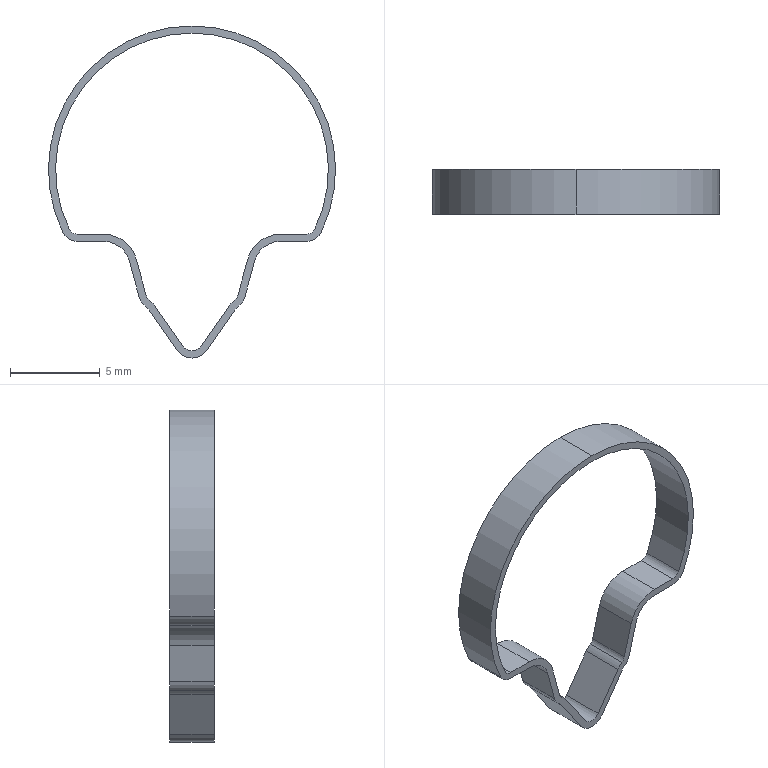Part | SolidWorks | features BaseBody 1 | 1 solid | 36 faces | box 16 x 2.5 x 18.5 mm | volume 53.347 mm3 | cylinder 22 | plane 14 | commonest cylinder face diameters 1 x4 1.8 x4 2 x3 2.8 x2 3 x2 3.8 x2
STEP:
#1=CARTESIAN_POINT('',(-7.197,-1.25,-3.493));
#2=VERTEX_POINT('',#1);
#3=CARTESIAN_POINT('',(0.,-1.25,8.));
#4=VERTEX_POINT('',#3);
#5=CARTESIAN_POINT('',(0.,-1.25,0.));
#6=DIRECTION('',(0.,1.,0.));
#7=DIRECTION('',(0.,0.,1.));
#8=AXIS2_PLACEMENT_3D('',#5,#6,#7);
#9=CIRCLE('',#8,8.);
#10=EDGE_CURVE('',#2,#4,#9,.T.);
#11=ORIENTED_EDGE('',*,*,#10,.T.);
#12=CARTESIAN_POINT('',(0.,1.25,8.));
#13=VERTEX_POINT('',#12);
#14=CARTESIAN_POINT('',(0.,-1.25,8.));
#15=DIRECTION('',(0.,1.,0.));
#16=VECTOR('',#15,1000.);
#17=LINE('',#14,#16);
#18=EDGE_CURVE('',#4,#13,#17,.T.);
#19=ORIENTED_EDGE('',*,*,#18,.T.);
#20=CARTESIAN_POINT('',(-7.197,1.25,-3.493));
#21=VERTEX_POINT('',#20);
#22=CARTESIAN_POINT('',(0.,1.25,0.));
#23=DIRECTION('',(0.,-1.,0.));
#24=DIRECTION('',(0.,0.,1.));
#25=AXIS2_PLACEMENT_3D('',#22,#23,#24);
#26=CIRCLE('',#25,8.);
#27=EDGE_CURVE('',#13,#21,#26,.T.);
#28=ORIENTED_EDGE('',*,*,#27,.T.);
#29=CARTESIAN_POINT('',(-7.197,-1.25,-3.493));
#30=DIRECTION('',(0.,-1.,0.));
#31=VECTOR('',#30,1000.);
#32=LINE('',#29,#31);
#33=EDGE_CURVE('',#21,#2,#32,.T.);
#34=ORIENTED_EDGE('',*,*,#33,.T.);
#35=EDGE_LOOP('',(#11,#19,#28,#34));
#36=FACE_OUTER_BOUND('',#35,.T.);
#37=CARTESIAN_POINT('',(0.,-1.25,0.));
#38=DIRECTION('',(0.,1.,0.));
#39=DIRECTION('',(0.,0.,1.));
#40=AXIS2_PLACEMENT_3D('',#37,#38,#39);
#41=CYLINDRICAL_SURFACE('',#40,8.);
#42=ADVANCED_FACE('',(#36),#41,.T.);
#43=CARTESIAN_POINT('',(6.837,-1.25,-3.318));
#44=VERTEX_POINT('',#43);
#45=CARTESIAN_POINT('',(0.,-1.25,7.6));
#46=VERTEX_POINT('',#45);
#47=CARTESIAN_POINT('',(0.,-1.25,0.));
#48=DIRECTION('',(0.,-1.,0.));
#49=DIRECTION('',(0.,0.,1.));
#50=AXIS2_PLACEMENT_3D('',#47,#48,#49);
#51=CIRCLE('',#50,7.6);
#52=EDGE_CURVE('',#44,#46,#51,.T.);
#53=ORIENTED_EDGE('',*,*,#52,.T.);
#54=CARTESIAN_POINT('',(0.,1.25,7.6));
#55=VERTEX_POINT('',#54);
#56=CARTESIAN_POINT('',(0.,-1.25,7.6));
#57=DIRECTION('',(0.,1.,0.));
#58=VECTOR('',#57,1000.);
#59=LINE('',#56,#58);
#60=EDGE_CURVE('',#46,#55,#59,.T.);
#61=ORIENTED_EDGE('',*,*,#60,.T.);
#62=CARTESIAN_POINT('',(6.837,1.25,-3.318));
#63=VERTEX_POINT('',#62);
#64=CARTESIAN_POINT('',(0.,1.25,0.));
#65=DIRECTION('',(0.,-1.,0.));
#66=DIRECTION('',(0.,0.,1.));
#67=AXIS2_PLACEMENT_3D('',#64,#65,#66);
#68=CIRCLE('',#67,7.6);
#69=EDGE_CURVE('',#63,#55,#68,.T.);
#70=ORIENTED_EDGE('',*,*,#69,.F.);
#71=CARTESIAN_POINT('',(6.837,-1.25,-3.318));
#72=DIRECTION('',(0.,1.,0.));
#73=VECTOR('',#72,1000.);
#74=LINE('',#71,#73);
#75=EDGE_CURVE('',#44,#63,#74,.T.);
#76=ORIENTED_EDGE('',*,*,#75,.F.);
#77=EDGE_LOOP('',(#53,#61,#70,#76));
#78=FACE_OUTER_BOUND('',#77,.T.);
#79=CARTESIAN_POINT('',(0.,-1.25,0.));
#80=DIRECTION('',(0.,1.,0.));
#81=DIRECTION('',(0.,0.,1.));
#82=AXIS2_PLACEMENT_3D('',#79,#80,#81);
#83=CYLINDRICAL_SURFACE('',#82,7.6);
#84=ADVANCED_FACE('',(#78),#83,.F.);
#85=ORIENTED_EDGE('',*,*,#18,.F.);
#86=CARTESIAN_POINT('',(7.197,-1.25,-3.493));
#87=VERTEX_POINT('',#86);
#88=CARTESIAN_POINT('',(0.,-1.25,0.));
#89=DIRECTION('',(0.,1.,0.));
#90=DIRECTION('',(0.,0.,1.));
#91=AXIS2_PLACEMENT_3D('',#88,#89,#90);
#92=CIRCLE('',#91,8.);
#93=EDGE_CURVE('',#4,#87,#92,.T.);
#94=ORIENTED_EDGE('',*,*,#93,.T.);
#95=CARTESIAN_POINT('',(7.197,1.25,-3.493));
#96=VERTEX_POINT('',#95);
#97=CARTESIAN_POINT('',(7.197,-1.25,-3.493));
#98=DIRECTION('',(0.,1.,0.));
#99=VECTOR('',#98,1000.);
#100=LINE('',#97,#99);
#101=EDGE_CURVE('',#87,#96,#100,.T.);
#102=ORIENTED_EDGE('',*,*,#101,.T.);
#103=CARTESIAN_POINT('',(0.,1.25,0.));
#104=DIRECTION('',(0.,-1.,0.));
#105=DIRECTION('',(0.,0.,1.));
#106=AXIS2_PLACEMENT_3D('',#103,#104,#105);
#107=CIRCLE('',#106,8.);
#108=EDGE_CURVE('',#96,#13,#107,.T.);
#109=ORIENTED_EDGE('',*,*,#108,.T.);
#110=EDGE_LOOP('',(#85,#94,#102,#109));
#111=FACE_OUTER_BOUND('',#110,.T.);
#112=CARTESIAN_POINT('',(0.,-1.25,0.));
#113=DIRECTION('',(0.,1.,0.));
#114=DIRECTION('',(0.,0.,1.));
#115=AXIS2_PLACEMENT_3D('',#112,#113,#114);
#116=CYLINDRICAL_SURFACE('',#115,8.);
#117=ADVANCED_FACE('',(#111),#116,.T.);
#118=CARTESIAN_POINT('',(6.387,-1.25,-4.));
#119=VERTEX_POINT('',#118);
#120=CARTESIAN_POINT('',(6.387,1.25,-4.));
#121=VERTEX_POINT('',#120);
#122=CARTESIAN_POINT('',(6.387,-4.509,-4.));
#123=DIRECTION('',(0.,1.,0.));
#124=VECTOR('',#123,1000.);
#125=LINE('',#122,#124);
#126=EDGE_CURVE('',#119,#121,#125,.T.);
#127=ORIENTED_EDGE('',*,*,#126,.T.);
#128=CARTESIAN_POINT('',(6.387,1.25,-3.1));
#129=DIRECTION('',(0.,-1.,0.));
#130=DIRECTION('',(0.,0.,1.));
#131=AXIS2_PLACEMENT_3D('',#128,#129,#130);
#132=CIRCLE('',#131,0.9);
#133=EDGE_CURVE('',#121,#96,#132,.T.);
#134=ORIENTED_EDGE('',*,*,#133,.T.);
#135=ORIENTED_EDGE('',*,*,#101,.F.);
#136=CARTESIAN_POINT('',(6.387,-1.25,-3.1));
#137=DIRECTION('',(0.,1.,0.));
#138=DIRECTION('',(0.,0.,1.));
#139=AXIS2_PLACEMENT_3D('',#136,#137,#138);
#140=CIRCLE('',#139,0.9);
#141=EDGE_CURVE('',#87,#119,#140,.T.);
#142=ORIENTED_EDGE('',*,*,#141,.T.);
#143=EDGE_LOOP('',(#127,#134,#135,#142));
#144=FACE_OUTER_BOUND('',#143,.T.);
#145=CARTESIAN_POINT('',(6.387,-4.509,-3.1));
#146=DIRECTION('',(0.,1.,0.));
#147=DIRECTION('',(0.,0.,1.));
#148=AXIS2_PLACEMENT_3D('',#145,#146,#147);
#149=CYLINDRICAL_SURFACE('',#148,0.9);
#150=ADVANCED_FACE('',(#144),#149,.T.);
#151=CARTESIAN_POINT('',(-4.931,-1.25,-3.6));
#152=VERTEX_POINT('',#151);
#153=CARTESIAN_POINT('',(-6.387,-1.25,-3.6));
#154=VERTEX_POINT('',#153);
#155=CARTESIAN_POINT('',(-7.144,-1.25,-3.6));
#156=DIRECTION('',(-1.,0.,0.));
#157=VECTOR('',#156,1000.);
#158=LINE('',#155,#157);
#159=EDGE_CURVE('',#152,#154,#158,.T.);
#160=ORIENTED_EDGE('',*,*,#159,.T.);
#161=CARTESIAN_POINT('',(-6.837,-1.25,-3.318));
#162=VERTEX_POINT('',#161);
#163=CARTESIAN_POINT('',(-6.387,-1.25,-3.1));
#164=DIRECTION('',(0.,1.,0.));
#165=DIRECTION('',(0.,0.,-1.));
#166=AXIS2_PLACEMENT_3D('',#163,#164,#165);
#167=CIRCLE('',#166,0.5);
#168=EDGE_CURVE('',#154,#162,#167,.T.);
#169=ORIENTED_EDGE('',*,*,#168,.T.);
#170=CARTESIAN_POINT('',(0.,-1.25,0.));
#171=DIRECTION('',(0.,-1.,0.));
#172=DIRECTION('',(0.,0.,1.));
#173=AXIS2_PLACEMENT_3D('',#170,#171,#172);
#174=CIRCLE('',#173,7.6);
#175=EDGE_CURVE('',#46,#162,#174,.T.);
#176=ORIENTED_EDGE('',*,*,#175,.F.);
#177=ORIENTED_EDGE('',*,*,#52,.F.);
#178=CARTESIAN_POINT('',(6.387,-1.25,-3.6));
#179=VERTEX_POINT('',#178);
#180=CARTESIAN_POINT('',(6.387,-1.25,-3.1));
#181=DIRECTION('',(0.,1.,0.));
#182=DIRECTION('',(0.,0.,1.));
#183=AXIS2_PLACEMENT_3D('',#180,#181,#182);
#184=CIRCLE('',#183,0.5);
#185=EDGE_CURVE('',#44,#179,#184,.T.);
#186=ORIENTED_EDGE('',*,*,#185,.T.);
#187=CARTESIAN_POINT('',(4.931,-1.25,-3.6));
#188=VERTEX_POINT('',#187);
#189=CARTESIAN_POINT('',(7.144,-1.25,-3.6));
#190=DIRECTION('',(1.,0.,0.));
#191=VECTOR('',#190,1000.);
#192=LINE('',#189,#191);
#193=EDGE_CURVE('',#188,#179,#192,.T.);
#194=ORIENTED_EDGE('',*,*,#193,.F.);
#195=CARTESIAN_POINT('',(3.096,-1.25,-5.008));
#196=VERTEX_POINT('',#195);
#197=CARTESIAN_POINT('',(4.931,-1.25,-5.5));
#198=DIRECTION('',(0.,1.,0.));
#199=DIRECTION('',(0.,0.,-1.));
#200=AXIS2_PLACEMENT_3D('',#197,#198,#199);
#201=CIRCLE('',#200,1.9);
#202=EDGE_CURVE('',#196,#188,#201,.T.);
#203=ORIENTED_EDGE('',*,*,#202,.F.);
#204=CARTESIAN_POINT('',(2.559,-1.25,-7.011));
#205=VERTEX_POINT('',#204);
#206=CARTESIAN_POINT('',(2.559,-1.25,-7.011));
#207=DIRECTION('',(0.2588,0.,0.9659));
#208=VECTOR('',#207,1000.);
#209=LINE('',#206,#208);
#210=EDGE_CURVE('',#205,#196,#209,.T.);
#211=ORIENTED_EDGE('',*,*,#210,.F.);
#212=CARTESIAN_POINT('',(2.373,-1.25,-7.284));
#213=VERTEX_POINT('',#212);
#214=CARTESIAN_POINT('',(2.076,-1.25,-6.882));
#215=DIRECTION('',(0.,1.,0.));
#216=DIRECTION('',(0.,0.,-1.));
#217=AXIS2_PLACEMENT_3D('',#214,#215,#216);
#218=CIRCLE('',#217,0.5);
#219=EDGE_CURVE('',#205,#213,#218,.T.);
#220=ORIENTED_EDGE('',*,*,#219,.T.);
#221=CARTESIAN_POINT('',(2.058,-1.25,-7.607));
#222=VERTEX_POINT('',#221);
#223=CARTESIAN_POINT('',(3.205,-1.25,-8.41));
#224=DIRECTION('',(0.,1.,0.));
#225=DIRECTION('',(0.,0.,1.));
#226=AXIS2_PLACEMENT_3D('',#223,#224,#225);
#227=CIRCLE('',#226,1.4);
#228=EDGE_CURVE('',#222,#213,#227,.T.);
#229=ORIENTED_EDGE('',*,*,#228,.F.);
#230=CARTESIAN_POINT('',(0.4915,-1.25,-9.844));
#231=VERTEX_POINT('',#230);
#232=CARTESIAN_POINT('',(0.4915,-1.25,-9.844));
#233=DIRECTION('',(0.5736,0.,0.8192));
#234=VECTOR('',#233,1000.);
#235=LINE('',#232,#234);
#236=EDGE_CURVE('',#231,#222,#235,.T.);
#237=ORIENTED_EDGE('',*,*,#236,.F.);
#238=CARTESIAN_POINT('',(-0.4915,-1.25,-9.844));
#239=VERTEX_POINT('',#238);
#240=CARTESIAN_POINT('',(0.,-1.25,-9.5));
#241=DIRECTION('',(0.,1.,0.));
#242=DIRECTION('',(0.,0.,1.));
#243=AXIS2_PLACEMENT_3D('',#240,#241,#242);
#244=CIRCLE('',#243,0.6);
#245=EDGE_CURVE('',#231,#239,#244,.T.);
#246=ORIENTED_EDGE('',*,*,#245,.T.);
#247=CARTESIAN_POINT('',(-2.058,-1.25,-7.607));
#248=VERTEX_POINT('',#247);
#249=CARTESIAN_POINT('',(-2.058,-1.25,-7.607));
#250=DIRECTION('',(0.5736,0.,-0.8192));
#251=VECTOR('',#250,1000.);
#252=LINE('',#249,#251);
#253=EDGE_CURVE('',#248,#239,#252,.T.);
#254=ORIENTED_EDGE('',*,*,#253,.F.);
#255=CARTESIAN_POINT('',(-2.373,-1.25,-7.284));
#256=VERTEX_POINT('',#255);
#257=CARTESIAN_POINT('',(-3.205,-1.25,-8.41));
#258=DIRECTION('',(0.,1.,0.));
#259=DIRECTION('',(0.,0.,1.));
#260=AXIS2_PLACEMENT_3D('',#257,#258,#259);
#261=CIRCLE('',#260,1.4);
#262=EDGE_CURVE('',#256,#248,#261,.T.);
#263=ORIENTED_EDGE('',*,*,#262,.F.);
#264=CARTESIAN_POINT('',(-2.559,-1.25,-7.011));
#265=VERTEX_POINT('',#264);
#266=CARTESIAN_POINT('',(-2.076,-1.25,-6.882));
#267=DIRECTION('',(0.,1.,0.));
#268=DIRECTION('',(0.,0.,1.));
#269=AXIS2_PLACEMENT_3D('',#266,#267,#268);
#270=CIRCLE('',#269,0.5);
#271=EDGE_CURVE('',#256,#265,#270,.T.);
#272=ORIENTED_EDGE('',*,*,#271,.T.);
#273=CARTESIAN_POINT('',(-3.096,-1.25,-5.008));
#274=VERTEX_POINT('',#273);
#275=CARTESIAN_POINT('',(-3.096,-1.25,-5.008));
#276=DIRECTION('',(0.2588,0.,-0.9659));
#277=VECTOR('',#276,1000.);
#278=LINE('',#275,#277);
#279=EDGE_CURVE('',#274,#265,#278,.T.);
#280=ORIENTED_EDGE('',*,*,#279,.F.);
#281=CARTESIAN_POINT('',(-4.931,-1.25,-5.5));
#282=DIRECTION('',(0.,1.,0.));
#283=DIRECTION('',(0.,0.,1.));
#284=AXIS2_PLACEMENT_3D('',#281,#282,#283);
#285=CIRCLE('',#284,1.9);
#286=EDGE_CURVE('',#152,#274,#285,.T.);
#287=ORIENTED_EDGE('',*,*,#286,.F.);
#288=EDGE_LOOP('',(#160,#169,#176,#177,#186,#194,#203,#211,#220,#229,#237,#246,#254,#263,#272,#280,#287));
#289=FACE_BOUND('',#288,.T.);
#290=CARTESIAN_POINT('',(-0.8192,-1.25,-10.074));
#291=VERTEX_POINT('',#290);
#292=CARTESIAN_POINT('',(-2.386,-1.25,-7.837));
#293=VERTEX_POINT('',#292);
#294=CARTESIAN_POINT('',(-0.8192,-1.25,-10.074));
#295=DIRECTION('',(-0.5736,0.,0.8192));
#296=VECTOR('',#295,1000.);
#297=LINE('',#294,#296);
#298=EDGE_CURVE('',#291,#293,#297,.T.);
#299=ORIENTED_EDGE('',*,*,#298,.F.);
#300=CARTESIAN_POINT('',(0.8192,-1.25,-10.074));
#301=VERTEX_POINT('',#300);
#302=CARTESIAN_POINT('',(0.,-1.25,-9.5));
#303=DIRECTION('',(0.,1.,0.));
#304=DIRECTION('',(0.,0.,1.));
#305=AXIS2_PLACEMENT_3D('',#302,#303,#304);
#306=CIRCLE('',#305,1.);
#307=EDGE_CURVE('',#301,#291,#306,.T.);
#308=ORIENTED_EDGE('',*,*,#307,.F.);
#309=CARTESIAN_POINT('',(2.386,-1.25,-7.837));
#310=VERTEX_POINT('',#309);
#311=CARTESIAN_POINT('',(2.386,-1.25,-7.837));
#312=DIRECTION('',(-0.5736,0.,-0.8192));
#313=VECTOR('',#312,1000.);
#314=LINE('',#311,#313);
#315=EDGE_CURVE('',#310,#301,#314,.T.);
#316=ORIENTED_EDGE('',*,*,#315,.F.);
#317=CARTESIAN_POINT('',(2.611,-1.25,-7.606));
#318=VERTEX_POINT('',#317);
#319=CARTESIAN_POINT('',(3.205,-1.25,-8.41));
#320=DIRECTION('',(0.,1.,0.));
#321=DIRECTION('',(0.,0.,1.));
#322=AXIS2_PLACEMENT_3D('',#319,#320,#321);
#323=CIRCLE('',#322,1.);
#324=EDGE_CURVE('',#310,#318,#323,.T.);
#325=ORIENTED_EDGE('',*,*,#324,.T.);
#326=CARTESIAN_POINT('',(2.945,-1.25,-7.115));
#327=VERTEX_POINT('',#326);
#328=CARTESIAN_POINT('',(2.076,-1.25,-6.882));
#329=DIRECTION('',(0.,1.,0.));
#330=DIRECTION('',(0.,0.,-1.));
#331=AXIS2_PLACEMENT_3D('',#328,#329,#330);
#332=CIRCLE('',#331,0.9);
#333=EDGE_CURVE('',#327,#318,#332,.T.);
#334=ORIENTED_EDGE('',*,*,#333,.F.);
#335=CARTESIAN_POINT('',(3.482,-1.25,-5.112));
#336=VERTEX_POINT('',#335);
#337=CARTESIAN_POINT('',(3.482,-1.25,-5.112));
#338=DIRECTION('',(-0.2588,0.,-0.9659));
#339=VECTOR('',#338,1000.);
#340=LINE('',#337,#339);
#341=EDGE_CURVE('',#336,#327,#340,.T.);
#342=ORIENTED_EDGE('',*,*,#341,.F.);
#343=CARTESIAN_POINT('',(4.931,-1.25,-4.));
#344=VERTEX_POINT('',#343);
#345=CARTESIAN_POINT('',(4.931,-1.25,-5.5));
#346=DIRECTION('',(0.,-1.,0.));
#347=DIRECTION('',(0.,0.,-1.));
#348=AXIS2_PLACEMENT_3D('',#345,#346,#347);
#349=CIRCLE('',#348,1.5);
#350=EDGE_CURVE('',#344,#336,#349,.T.);
#351=ORIENTED_EDGE('',*,*,#350,.F.);
#352=CARTESIAN_POINT('',(0.,-1.25,-4.));
#353=DIRECTION('',(-1.,0.,0.));
#354=VECTOR('',#353,1000.);
#355=LINE('',#352,#354);
#356=EDGE_CURVE('',#119,#344,#355,.T.);
#357=ORIENTED_EDGE('',*,*,#356,.F.);
#358=ORIENTED_EDGE('',*,*,#141,.F.);
#359=ORIENTED_EDGE('',*,*,#93,.F.);
#360=ORIENTED_EDGE('',*,*,#10,.F.);
#361=CARTESIAN_POINT('',(-6.387,-1.25,-4.));
#362=VERTEX_POINT('',#361);
#363=CARTESIAN_POINT('',(-6.387,-1.25,-3.1));
#364=DIRECTION('',(0.,1.,0.));
#365=DIRECTION('',(0.,0.,-1.));
#366=AXIS2_PLACEMENT_3D('',#363,#364,#365);
#367=CIRCLE('',#366,0.9);
#368=EDGE_CURVE('',#362,#2,#367,.T.);
#369=ORIENTED_EDGE('',*,*,#368,.F.);
#370=CARTESIAN_POINT('',(-4.931,-1.25,-4.));
#371=VERTEX_POINT('',#370);
#372=CARTESIAN_POINT('',(-4.931,-1.25,-4.));
#373=DIRECTION('',(1.,0.,0.));
#374=VECTOR('',#373,1000.);
#375=LINE('',#372,#374);
#376=EDGE_CURVE('',#362,#371,#375,.T.);
#377=ORIENTED_EDGE('',*,*,#376,.T.);
#378=CARTESIAN_POINT('',(-3.482,-1.25,-5.112));
#379=VERTEX_POINT('',#378);
#380=CARTESIAN_POINT('',(-4.931,-1.25,-5.5));
#381=DIRECTION('',(0.,-1.,0.));
#382=DIRECTION('',(0.,0.,1.));
#383=AXIS2_PLACEMENT_3D('',#380,#381,#382);
#384=CIRCLE('',#383,1.5);
#385=EDGE_CURVE('',#379,#371,#384,.T.);
#386=ORIENTED_EDGE('',*,*,#385,.F.);
#387=CARTESIAN_POINT('',(-2.945,-1.25,-7.115));
#388=VERTEX_POINT('',#387);
#389=CARTESIAN_POINT('',(-2.945,-1.25,-7.115));
#390=DIRECTION('',(-0.2588,0.,0.9659));
#391=VECTOR('',#390,1000.);
#392=LINE('',#389,#391);
#393=EDGE_CURVE('',#388,#379,#392,.T.);
#394=ORIENTED_EDGE('',*,*,#393,.F.);
#395=CARTESIAN_POINT('',(-2.611,-1.25,-7.606));
#396=VERTEX_POINT('',#395);
#397=CARTESIAN_POINT('',(-2.076,-1.25,-6.882));
#398=DIRECTION('',(0.,1.,0.));
#399=DIRECTION('',(0.,0.,1.));
#400=AXIS2_PLACEMENT_3D('',#397,#398,#399);
#401=CIRCLE('',#400,0.9);
#402=EDGE_CURVE('',#396,#388,#401,.T.);
#403=ORIENTED_EDGE('',*,*,#402,.F.);
#404=CARTESIAN_POINT('',(-3.205,-1.25,-8.41));
#405=DIRECTION('',(0.,1.,0.));
#406=DIRECTION('',(0.,0.,1.));
#407=AXIS2_PLACEMENT_3D('',#404,#405,#406);
#408=CIRCLE('',#407,1.);
#409=EDGE_CURVE('',#396,#293,#408,.T.);
#410=ORIENTED_EDGE('',*,*,#409,.T.);
#411=EDGE_LOOP('',(#299,#308,#316,#325,#334,#342,#351,#357,#358,#359,#360,#369,#377,#386,#394,#403,#410));
#412=FACE_OUTER_BOUND('',#411,.T.);
#413=CARTESIAN_POINT('',(0.,-1.25,0.));
#414=DIRECTION('',(0.,1.,0.));
#415=DIRECTION('',(0.,0.,1.));
#416=AXIS2_PLACEMENT_3D('',#413,#414,#415);
#417=PLANE('',#416);
#418=ADVANCED_FACE('',(#289,#412),#417,.F.);
#419=CARTESIAN_POINT('',(-6.387,1.25,-4.));
#420=VERTEX_POINT('',#419);
#421=CARTESIAN_POINT('',(-6.387,4.509,-4.));
#422=DIRECTION('',(0.,-1.,0.));
#423=VECTOR('',#422,1000.);
#424=LINE('',#421,#423);
#425=EDGE_CURVE('',#420,#362,#424,.T.);
#426=ORIENTED_EDGE('',*,*,#425,.T.);
#427=ORIENTED_EDGE('',*,*,#368,.T.);
#428=ORIENTED_EDGE('',*,*,#33,.F.);
#429=CARTESIAN_POINT('',(-6.387,1.25,-3.1));
#430=DIRECTION('',(0.,-1.,0.));
#431=DIRECTION('',(0.,0.,-1.));
#432=AXIS2_PLACEMENT_3D('',#429,#430,#431);
#433=CIRCLE('',#432,0.9);
#434=EDGE_CURVE('',#21,#420,#433,.T.);
#435=ORIENTED_EDGE('',*,*,#434,.T.);
#436=EDGE_LOOP('',(#426,#427,#428,#435));
#437=FACE_OUTER_BOUND('',#436,.T.);
#438=CARTESIAN_POINT('',(-6.387,4.509,-3.1));
#439=DIRECTION('',(0.,-1.,0.));
#440=DIRECTION('',(0.,0.,-1.));
#441=AXIS2_PLACEMENT_3D('',#438,#439,#440);
#442=CYLINDRICAL_SURFACE('',#441,0.9);
#443=ADVANCED_FACE('',(#437),#442,.T.);
#444=CARTESIAN_POINT('',(-2.559,1.25,-7.011));
#445=VERTEX_POINT('',#444);
#446=CARTESIAN_POINT('',(-2.373,1.25,-7.284));
#447=VERTEX_POINT('',#446);
#448=CARTESIAN_POINT('',(-2.076,1.25,-6.882));
#449=DIRECTION('',(0.,-1.,0.));
#450=DIRECTION('',(0.,0.,1.));
#451=AXIS2_PLACEMENT_3D('',#448,#449,#450);
#452=CIRCLE('',#451,0.5);
#453=EDGE_CURVE('',#445,#447,#452,.T.);
#454=ORIENTED_EDGE('',*,*,#453,.T.);
#455=CARTESIAN_POINT('',(-2.058,1.25,-7.607));
#456=VERTEX_POINT('',#455);
#457=CARTESIAN_POINT('',(-3.205,1.25,-8.41));
#458=DIRECTION('',(0.,-1.,0.));
#459=DIRECTION('',(0.,0.,1.));
#460=AXIS2_PLACEMENT_3D('',#457,#458,#459);
#461=CIRCLE('',#460,1.4);
#462=EDGE_CURVE('',#456,#447,#461,.T.);
#463=ORIENTED_EDGE('',*,*,#462,.F.);
#464=CARTESIAN_POINT('',(-0.4915,1.25,-9.844));
#465=VERTEX_POINT('',#464);
#466=CARTESIAN_POINT('',(-2.058,1.25,-7.607));
#467=DIRECTION('',(0.5736,0.,-0.8192));
#468=VECTOR('',#467,1000.);
#469=LINE('',#466,#468);
#470=EDGE_CURVE('',#456,#465,#469,.T.);
#471=ORIENTED_EDGE('',*,*,#470,.T.);
#472=CARTESIAN_POINT('',(0.4915,1.25,-9.844));
#473=VERTEX_POINT('',#472);
#474=CARTESIAN_POINT('',(0.,1.25,-9.5));
#475=DIRECTION('',(0.,-1.,0.));
#476=DIRECTION('',(0.,0.,1.));
#477=AXIS2_PLACEMENT_3D('',#474,#475,#476);
#478=CIRCLE('',#477,0.6);
#479=EDGE_CURVE('',#465,#473,#478,.T.);
#480=ORIENTED_EDGE('',*,*,#479,.T.);
#481=CARTESIAN_POINT('',(2.058,1.25,-7.607));
#482=VERTEX_POINT('',#481);
#483=CARTESIAN_POINT('',(0.4915,1.25,-9.844));
#484=DIRECTION('',(0.5736,0.,0.8192));
#485=VECTOR('',#484,1000.);
#486=LINE('',#483,#485);
#487=EDGE_CURVE('',#473,#482,#486,.T.);
#488=ORIENTED_EDGE('',*,*,#487,.T.);
#489=CARTESIAN_POINT('',(2.373,1.25,-7.284));
#490=VERTEX_POINT('',#489);
#491=CARTESIAN_POINT('',(3.205,1.25,-8.41));
#492=DIRECTION('',(0.,-1.,0.));
#493=DIRECTION('',(0.,0.,1.));
#494=AXIS2_PLACEMENT_3D('',#491,#492,#493);
#495=CIRCLE('',#494,1.4);
#496=EDGE_CURVE('',#490,#482,#495,.T.);
#497=ORIENTED_EDGE('',*,*,#496,.F.);
#498=CARTESIAN_POINT('',(2.559,1.25,-7.011));
#499=VERTEX_POINT('',#498);
#500=CARTESIAN_POINT('',(2.076,1.25,-6.882));
#501=DIRECTION('',(0.,-1.,0.));
#502=DIRECTION('',(0.,0.,-1.));
#503=AXIS2_PLACEMENT_3D('',#500,#501,#502);
#504=CIRCLE('',#503,0.5);
#505=EDGE_CURVE('',#490,#499,#504,.T.);
#506=ORIENTED_EDGE('',*,*,#505,.T.);
#507=CARTESIAN_POINT('',(3.096,1.25,-5.008));
#508=VERTEX_POINT('',#507);
#509=CARTESIAN_POINT('',(2.559,1.25,-7.011));
#510=DIRECTION('',(0.2588,0.,0.9659));
#511=VECTOR('',#510,1000.);
#512=LINE('',#509,#511);
#513=EDGE_CURVE('',#499,#508,#512,.T.);
#514=ORIENTED_EDGE('',*,*,#513,.T.);
#515=CARTESIAN_POINT('',(4.931,1.25,-3.6));
#516=VERTEX_POINT('',#515);
#517=CARTESIAN_POINT('',(4.931,1.25,-5.5));
#518=DIRECTION('',(0.,1.,0.));
#519=DIRECTION('',(0.,0.,-1.));
#520=AXIS2_PLACEMENT_3D('',#517,#518,#519);
#521=CIRCLE('',#520,1.9);
#522=EDGE_CURVE('',#508,#516,#521,.T.);
#523=ORIENTED_EDGE('',*,*,#522,.T.);
#524=CARTESIAN_POINT('',(6.387,1.25,-3.6));
#525=VERTEX_POINT('',#524);
#526=CARTESIAN_POINT('',(7.144,1.25,-3.6));
#527=DIRECTION('',(-1.,0.,0.));
#528=VECTOR('',#527,1000.);
#529=LINE('',#526,#528);
#530=EDGE_CURVE('',#525,#516,#529,.T.);
#531=ORIENTED_EDGE('',*,*,#530,.F.);
#532=CARTESIAN_POINT('',(6.387,1.25,-3.1));
#533=DIRECTION('',(0.,-1.,0.));
#534=DIRECTION('',(0.,0.,1.));
#535=AXIS2_PLACEMENT_3D('',#532,#533,#534);
#536=CIRCLE('',#535,0.5);
#537=EDGE_CURVE('',#525,#63,#536,.T.);
#538=ORIENTED_EDGE('',*,*,#537,.T.);
#539=ORIENTED_EDGE('',*,*,#69,.T.);
#540=CARTESIAN_POINT('',(-6.837,1.25,-3.318));
#541=VERTEX_POINT('',#540);
#542=CARTESIAN_POINT('',(0.,1.25,0.));
#543=DIRECTION('',(0.,-1.,0.));
#544=DIRECTION('',(0.,0.,1.));
#545=AXIS2_PLACEMENT_3D('',#542,#543,#544);
#546=CIRCLE('',#545,7.6);
#547=EDGE_CURVE('',#55,#541,#546,.T.);
#548=ORIENTED_EDGE('',*,*,#547,.T.);
#549=CARTESIAN_POINT('',(-6.387,1.25,-3.6));
#550=VERTEX_POINT('',#549);
#551=CARTESIAN_POINT('',(-6.387,1.25,-3.1));
#552=DIRECTION('',(0.,-1.,0.));
#553=DIRECTION('',(0.,0.,-1.));
#554=AXIS2_PLACEMENT_3D('',#551,#552,#553);
#555=CIRCLE('',#554,0.5);
#556=EDGE_CURVE('',#541,#550,#555,.T.);
#557=ORIENTED_EDGE('',*,*,#556,.T.);
#558=CARTESIAN_POINT('',(-4.931,1.25,-3.6));
#559=VERTEX_POINT('',#558);
#560=CARTESIAN_POINT('',(-7.144,1.25,-3.6));
#561=DIRECTION('',(1.,0.,0.));
#562=VECTOR('',#561,1000.);
#563=LINE('',#560,#562);
#564=EDGE_CURVE('',#550,#559,#563,.T.);
#565=ORIENTED_EDGE('',*,*,#564,.T.);
#566=CARTESIAN_POINT('',(-3.096,1.25,-5.008));
#567=VERTEX_POINT('',#566);
#568=CARTESIAN_POINT('',(-4.931,1.25,-5.5));
#569=DIRECTION('',(0.,1.,0.));
#570=DIRECTION('',(0.,0.,1.));
#571=AXIS2_PLACEMENT_3D('',#568,#569,#570);
#572=CIRCLE('',#571,1.9);
#573=EDGE_CURVE('',#559,#567,#572,.T.);
#574=ORIENTED_EDGE('',*,*,#573,.T.);
#575=CARTESIAN_POINT('',(-3.096,1.25,-5.008));
#576=DIRECTION('',(0.2588,0.,-0.9659));
#577=VECTOR('',#576,1000.);
#578=LINE('',#575,#577);
#579=EDGE_CURVE('',#567,#445,#578,.T.);
#580=ORIENTED_EDGE('',*,*,#579,.T.);
#581=EDGE_LOOP('',(#454,#463,#471,#480,#488,#497,#506,#514,#523,#531,#538,#539,#548,#557,#565,#574,#580));
#582=FACE_BOUND('',#581,.T.);
#583=CARTESIAN_POINT('',(-2.386,1.25,-7.837));
#584=VERTEX_POINT('',#583);
#585=CARTESIAN_POINT('',(-2.611,1.25,-7.606));
#586=VERTEX_POINT('',#585);
#587=CARTESIAN_POINT('',(-3.205,1.25,-8.41));
#588=DIRECTION('',(0.,-1.,0.));
#589=DIRECTION('',(0.,0.,1.));
#590=AXIS2_PLACEMENT_3D('',#587,#588,#589);
#591=CIRCLE('',#590,1.);
#592=EDGE_CURVE('',#584,#586,#591,.T.);
#593=ORIENTED_EDGE('',*,*,#592,.T.);
#594=CARTESIAN_POINT('',(-2.945,1.25,-7.115));
#595=VERTEX_POINT('',#594);
#596=CARTESIAN_POINT('',(-2.076,1.25,-6.882));
#597=DIRECTION('',(0.,-1.,0.));
#598=DIRECTION('',(0.,0.,1.));
#599=AXIS2_PLACEMENT_3D('',#596,#597,#598);
#600=CIRCLE('',#599,0.9);
#601=EDGE_CURVE('',#595,#586,#600,.T.);
#602=ORIENTED_EDGE('',*,*,#601,.F.);
#603=CARTESIAN_POINT('',(-3.482,1.25,-5.112));
#604=VERTEX_POINT('',#603);
#605=CARTESIAN_POINT('',(-2.945,1.25,-7.115));
#606=DIRECTION('',(-0.2588,0.,0.9659));
#607=VECTOR('',#606,1000.);
#608=LINE('',#605,#607);
#609=EDGE_CURVE('',#595,#604,#608,.T.);
#610=ORIENTED_EDGE('',*,*,#609,.T.);
#611=CARTESIAN_POINT('',(-4.931,1.25,-4.));
#612=VERTEX_POINT('',#611);
#613=CARTESIAN_POINT('',(-4.931,1.25,-5.5));
#614=DIRECTION('',(0.,-1.,0.));
#615=DIRECTION('',(0.,0.,1.));
#616=AXIS2_PLACEMENT_3D('',#613,#614,#615);
#617=CIRCLE('',#616,1.5);
#618=EDGE_CURVE('',#604,#612,#617,.T.);
#619=ORIENTED_EDGE('',*,*,#618,.T.);
#620=CARTESIAN_POINT('',(0.,1.25,-4.));
#621=DIRECTION('',(-1.,0.,0.));
#622=VECTOR('',#621,1000.);
#623=LINE('',#620,#622);
#624=EDGE_CURVE('',#612,#420,#623,.T.);
#625=ORIENTED_EDGE('',*,*,#624,.T.);
#626=ORIENTED_EDGE('',*,*,#434,.F.);
#627=ORIENTED_EDGE('',*,*,#27,.F.);
#628=ORIENTED_EDGE('',*,*,#108,.F.);
#629=ORIENTED_EDGE('',*,*,#133,.F.);
#630=CARTESIAN_POINT('',(4.931,1.25,-4.));
#631=VERTEX_POINT('',#630);
#632=CARTESIAN_POINT('',(0.,1.25,-4.));
#633=DIRECTION('',(-1.,0.,0.));
#634=VECTOR('',#633,1000.);
#635=LINE('',#632,#634);
#636=EDGE_CURVE('',#121,#631,#635,.T.);
#637=ORIENTED_EDGE('',*,*,#636,.T.);
#638=CARTESIAN_POINT('',(3.482,1.25,-5.112));
#639=VERTEX_POINT('',#638);
#640=CARTESIAN_POINT('',(4.931,1.25,-5.5));
#641=DIRECTION('',(0.,-1.,0.));
#642=DIRECTION('',(0.,0.,-1.));
#643=AXIS2_PLACEMENT_3D('',#640,#641,#642);
#644=CIRCLE('',#643,1.5);
#645=EDGE_CURVE('',#631,#639,#644,.T.);
#646=ORIENTED_EDGE('',*,*,#645,.T.);
#647=CARTESIAN_POINT('',(2.945,1.25,-7.115));
#648=VERTEX_POINT('',#647);
#649=CARTESIAN_POINT('',(3.482,1.25,-5.112));
#650=DIRECTION('',(-0.2588,0.,-0.9659));
#651=VECTOR('',#650,1000.);
#652=LINE('',#649,#651);
#653=EDGE_CURVE('',#639,#648,#652,.T.);
#654=ORIENTED_EDGE('',*,*,#653,.T.);
#655=CARTESIAN_POINT('',(2.611,1.25,-7.606));
#656=VERTEX_POINT('',#655);
#657=CARTESIAN_POINT('',(2.076,1.25,-6.882));
#658=DIRECTION('',(0.,-1.,0.));
#659=DIRECTION('',(0.,0.,-1.));
#660=AXIS2_PLACEMENT_3D('',#657,#658,#659);
#661=CIRCLE('',#660,0.9);
#662=EDGE_CURVE('',#656,#648,#661,.T.);
#663=ORIENTED_EDGE('',*,*,#662,.F.);
#664=CARTESIAN_POINT('',(2.386,1.25,-7.837));
#665=VERTEX_POINT('',#664);
#666=CARTESIAN_POINT('',(3.205,1.25,-8.41));
#667=DIRECTION('',(0.,-1.,0.));
#668=DIRECTION('',(0.,0.,1.));
#669=AXIS2_PLACEMENT_3D('',#666,#667,#668);
#670=CIRCLE('',#669,1.);
#671=EDGE_CURVE('',#656,#665,#670,.T.);
#672=ORIENTED_EDGE('',*,*,#671,.T.);
#673=CARTESIAN_POINT('',(0.8192,1.25,-10.074));
#674=VERTEX_POINT('',#673);
#675=CARTESIAN_POINT('',(2.386,1.25,-7.837));
#676=DIRECTION('',(-0.5736,0.,-0.8192));
#677=VECTOR('',#676,1000.);
#678=LINE('',#675,#677);
#679=EDGE_CURVE('',#665,#674,#678,.T.);
#680=ORIENTED_EDGE('',*,*,#679,.T.);
#681=CARTESIAN_POINT('',(-0.8192,1.25,-10.074));
#682=VERTEX_POINT('',#681);
#683=CARTESIAN_POINT('',(0.,1.25,-9.5));
#684=DIRECTION('',(0.,1.,0.));
#685=DIRECTION('',(0.,0.,1.));
#686=AXIS2_PLACEMENT_3D('',#683,#684,#685);
#687=CIRCLE('',#686,1.);
#688=EDGE_CURVE('',#674,#682,#687,.T.);
#689=ORIENTED_EDGE('',*,*,#688,.T.);
#690=CARTESIAN_POINT('',(-0.8192,1.25,-10.074));
#691=DIRECTION('',(-0.5736,0.,0.8192));
#692=VECTOR('',#691,1000.);
#693=LINE('',#690,#692);
#694=EDGE_CURVE('',#682,#584,#693,.T.);
#695=ORIENTED_EDGE('',*,*,#694,.T.);
#696=EDGE_LOOP('',(#593,#602,#610,#619,#625,#626,#627,#628,#629,#637,#646,#654,#663,#672,#680,#689,#695));
#697=FACE_OUTER_BOUND('',#696,.T.);
#698=CARTESIAN_POINT('',(0.,1.25,0.));
#699=DIRECTION('',(0.,1.,0.));
#700=DIRECTION('',(0.,0.,1.));
#701=AXIS2_PLACEMENT_3D('',#698,#699,#700);
#702=PLANE('',#701);
#703=ADVANCED_FACE('',(#582,#697),#702,.T.);
#704=ORIENTED_EDGE('',*,*,#636,.F.);
#705=ORIENTED_EDGE('',*,*,#126,.F.);
#706=ORIENTED_EDGE('',*,*,#356,.T.);
#707=CARTESIAN_POINT('',(4.931,-1.25,-4.));
#708=DIRECTION('',(0.,1.,0.));
#709=VECTOR('',#708,1000.);
#710=LINE('',#707,#709);
#711=EDGE_CURVE('',#344,#631,#710,.T.);
#712=ORIENTED_EDGE('',*,*,#711,.T.);
#713=EDGE_LOOP('',(#704,#705,#706,#712));
#714=FACE_OUTER_BOUND('',#713,.T.);
#715=CARTESIAN_POINT('',(4.931,-1.25,-4.));
#716=DIRECTION('',(0.,0.,-1.));
#717=DIRECTION('',(-1.,0.,0.));
#718=AXIS2_PLACEMENT_3D('',#715,#716,#717);
#719=PLANE('',#718);
#720=ADVANCED_FACE('',(#714),#719,.T.);
#721=CARTESIAN_POINT('',(-4.931,-1.25,-3.6));
#722=DIRECTION('',(0.,-1.,0.));
#723=VECTOR('',#722,1000.);
#724=LINE('',#721,#723);
#725=EDGE_CURVE('',#559,#152,#724,.T.);
#726=ORIENTED_EDGE('',*,*,#725,.T.);
#727=ORIENTED_EDGE('',*,*,#286,.T.);
#728=CARTESIAN_POINT('',(-3.096,-1.25,-5.008));
#729=DIRECTION('',(0.,1.,0.));
#730=VECTOR('',#729,1000.);
#731=LINE('',#728,#730);
#732=EDGE_CURVE('',#274,#567,#731,.T.);
#733=ORIENTED_EDGE('',*,*,#732,.T.);
#734=ORIENTED_EDGE('',*,*,#573,.F.);
#735=EDGE_LOOP('',(#726,#727,#733,#734));
#736=FACE_OUTER_BOUND('',#735,.T.);
#737=CARTESIAN_POINT('',(-4.931,-1.25,-5.5));
#738=DIRECTION('',(0.,1.,0.));
#739=DIRECTION('',(0.,0.,1.));
#740=AXIS2_PLACEMENT_3D('',#737,#738,#739);
#741=CYLINDRICAL_SURFACE('',#740,1.9);
#742=ADVANCED_FACE('',(#736),#741,.T.);
#743=ORIENTED_EDGE('',*,*,#60,.F.);
#744=ORIENTED_EDGE('',*,*,#175,.T.);
#745=CARTESIAN_POINT('',(-6.837,-1.25,-3.318));
#746=DIRECTION('',(0.,-1.,0.));
#747=VECTOR('',#746,1000.);
#748=LINE('',#745,#747);
#749=EDGE_CURVE('',#541,#162,#748,.T.);
#750=ORIENTED_EDGE('',*,*,#749,.F.);
#751=ORIENTED_EDGE('',*,*,#547,.F.);
#752=EDGE_LOOP('',(#743,#744,#750,#751));
#753=FACE_OUTER_BOUND('',#752,.T.);
#754=CARTESIAN_POINT('',(0.,-1.25,0.));
#755=DIRECTION('',(0.,1.,0.));
#756=DIRECTION('',(0.,0.,1.));
#757=AXIS2_PLACEMENT_3D('',#754,#755,#756);
#758=CYLINDRICAL_SURFACE('',#757,7.6);
#759=ADVANCED_FACE('',(#753),#758,.F.);
#760=CARTESIAN_POINT('',(3.096,-1.25,-5.008));
#761=DIRECTION('',(0.,-1.,0.));
#762=VECTOR('',#761,1000.);
#763=LINE('',#760,#762);
#764=EDGE_CURVE('',#508,#196,#763,.T.);
#765=ORIENTED_EDGE('',*,*,#764,.T.);
#766=ORIENTED_EDGE('',*,*,#202,.T.);
#767=CARTESIAN_POINT('',(4.931,-1.25,-3.6));
#768=DIRECTION('',(0.,1.,0.));
#769=VECTOR('',#768,1000.);
#770=LINE('',#767,#769);
#771=EDGE_CURVE('',#188,#516,#770,.T.);
#772=ORIENTED_EDGE('',*,*,#771,.T.);
#773=ORIENTED_EDGE('',*,*,#522,.F.);
#774=EDGE_LOOP('',(#765,#766,#772,#773));
#775=FACE_OUTER_BOUND('',#774,.T.);
#776=CARTESIAN_POINT('',(4.931,-1.25,-5.5));
#777=DIRECTION('',(0.,-1.,0.));
#778=DIRECTION('',(0.,0.,-1.));
#779=AXIS2_PLACEMENT_3D('',#776,#777,#778);
#780=CYLINDRICAL_SURFACE('',#779,1.9);
#781=ADVANCED_FACE('',(#775),#780,.T.);
#782=ORIENTED_EDGE('',*,*,#513,.F.);
#783=CARTESIAN_POINT('',(2.559,-1.25,-7.011));
#784=DIRECTION('',(0.,-1.,0.));
#785=VECTOR('',#784,1000.);
#786=LINE('',#783,#785);
#787=EDGE_CURVE('',#499,#205,#786,.T.);
#788=ORIENTED_EDGE('',*,*,#787,.T.);
#789=ORIENTED_EDGE('',*,*,#210,.T.);
#790=ORIENTED_EDGE('',*,*,#764,.F.);
#791=EDGE_LOOP('',(#782,#788,#789,#790));
#792=FACE_OUTER_BOUND('',#791,.T.);
#793=CARTESIAN_POINT('',(3.096,-1.25,-5.008));
#794=DIRECTION('',(-0.9659,0.,0.2588));
#795=DIRECTION('',(0.2588,0.,0.9659));
#796=AXIS2_PLACEMENT_3D('',#793,#794,#795);
#797=PLANE('',#796);
#798=ADVANCED_FACE('',(#792),#797,.T.);
#799=CARTESIAN_POINT('',(0.4915,-1.25,-9.844));
#800=DIRECTION('',(0.,-1.,0.));
#801=VECTOR('',#800,1000.);
#802=LINE('',#799,#801);
#803=EDGE_CURVE('',#473,#231,#802,.T.);
#804=ORIENTED_EDGE('',*,*,#803,.T.);
#805=ORIENTED_EDGE('',*,*,#236,.T.);
#806=CARTESIAN_POINT('',(2.058,-1.25,-7.607));
#807=DIRECTION('',(0.,1.,0.));
#808=VECTOR('',#807,1000.);
#809=LINE('',#806,#808);
#810=EDGE_CURVE('',#222,#482,#809,.T.);
#811=ORIENTED_EDGE('',*,*,#810,.T.);
#812=ORIENTED_EDGE('',*,*,#487,.F.);
#813=EDGE_LOOP('',(#804,#805,#811,#812));
#814=FACE_OUTER_BOUND('',#813,.T.);
#815=CARTESIAN_POINT('',(0.4915,-1.25,-9.844));
#816=DIRECTION('',(-0.8192,0.,0.5736));
#817=DIRECTION('',(0.5736,0.,0.8192));
#818=AXIS2_PLACEMENT_3D('',#815,#816,#817);
#819=PLANE('',#818);
#820=ADVANCED_FACE('',(#814),#819,.T.);
#821=CARTESIAN_POINT('',(-2.058,-1.25,-7.607));
#822=DIRECTION('',(0.,-1.,0.));
#823=VECTOR('',#822,1000.);
#824=LINE('',#821,#823);
#825=EDGE_CURVE('',#456,#248,#824,.T.);
#826=ORIENTED_EDGE('',*,*,#825,.T.);
#827=ORIENTED_EDGE('',*,*,#253,.T.);
#828=CARTESIAN_POINT('',(-0.4915,-1.25,-9.844));
#829=DIRECTION('',(0.,1.,0.));
#830=VECTOR('',#829,1000.);
#831=LINE('',#828,#830);
#832=EDGE_CURVE('',#239,#465,#831,.T.);
#833=ORIENTED_EDGE('',*,*,#832,.T.);
#834=ORIENTED_EDGE('',*,*,#470,.F.);
#835=EDGE_LOOP('',(#826,#827,#833,#834));
#836=FACE_OUTER_BOUND('',#835,.T.);
#837=CARTESIAN_POINT('',(-2.058,-1.25,-7.607));
#838=DIRECTION('',(0.8192,0.,0.5736));
#839=DIRECTION('',(0.5736,0.,-0.8192));
#840=AXIS2_PLACEMENT_3D('',#837,#838,#839);
#841=PLANE('',#840);
#842=ADVANCED_FACE('',(#836),#841,.T.);
#843=ORIENTED_EDGE('',*,*,#732,.F.);
#844=ORIENTED_EDGE('',*,*,#279,.T.);
#845=CARTESIAN_POINT('',(-2.559,-1.25,-7.011));
#846=DIRECTION('',(0.,-1.,0.));
#847=VECTOR('',#846,1000.);
#848=LINE('',#845,#847);
#849=EDGE_CURVE('',#445,#265,#848,.T.);
#850=ORIENTED_EDGE('',*,*,#849,.F.);
#851=ORIENTED_EDGE('',*,*,#579,.F.);
#852=EDGE_LOOP('',(#843,#844,#850,#851));
#853=FACE_OUTER_BOUND('',#852,.T.);
#854=CARTESIAN_POINT('',(-3.096,-1.25,-5.008));
#855=DIRECTION('',(-0.9659,0.,-0.2588));
#856=DIRECTION('',(-0.2588,0.,0.9659));
#857=AXIS2_PLACEMENT_3D('',#854,#855,#856);
#858=PLANE('',#857);
#859=ADVANCED_FACE('',(#853),#858,.F.);
#860=CARTESIAN_POINT('',(-0.8192,-1.25,-10.074));
#861=DIRECTION('',(0.,-1.,0.));
#862=VECTOR('',#861,1000.);
#863=LINE('',#860,#862);
#864=EDGE_CURVE('',#682,#291,#863,.T.);
#865=ORIENTED_EDGE('',*,*,#864,.T.);
#866=ORIENTED_EDGE('',*,*,#298,.T.);
#867=CARTESIAN_POINT('',(-2.386,-1.25,-7.837));
#868=DIRECTION('',(0.,1.,0.));
#869=VECTOR('',#868,1000.);
#870=LINE('',#867,#869);
#871=EDGE_CURVE('',#293,#584,#870,.T.);
#872=ORIENTED_EDGE('',*,*,#871,.T.);
#873=ORIENTED_EDGE('',*,*,#694,.F.);
#874=EDGE_LOOP('',(#865,#866,#872,#873));
#875=FACE_OUTER_BOUND('',#874,.T.);
#876=CARTESIAN_POINT('',(-0.8192,-1.25,-10.074));
#877=DIRECTION('',(-0.8192,0.,-0.5736));
#878=DIRECTION('',(-0.5736,0.,0.8192));
#879=AXIS2_PLACEMENT_3D('',#876,#877,#878);
#880=PLANE('',#879);
#881=ADVANCED_FACE('',(#875),#880,.T.);
#882=CARTESIAN_POINT('',(0.8192,-1.25,-10.074));
#883=DIRECTION('',(0.,-1.,0.));
#884=VECTOR('',#883,1000.);
#885=LINE('',#882,#884);
#886=EDGE_CURVE('',#674,#301,#885,.T.);
#887=ORIENTED_EDGE('',*,*,#886,.T.);
#888=ORIENTED_EDGE('',*,*,#307,.T.);
#889=ORIENTED_EDGE('',*,*,#864,.F.);
#890=ORIENTED_EDGE('',*,*,#688,.F.);
#891=EDGE_LOOP('',(#887,#888,#889,#890));
#892=FACE_OUTER_BOUND('',#891,.T.);
#893=CARTESIAN_POINT('',(0.,-1.25,-9.5));
#894=DIRECTION('',(0.,1.,0.));
#895=DIRECTION('',(0.,0.,1.));
#896=AXIS2_PLACEMENT_3D('',#893,#894,#895);
#897=CYLINDRICAL_SURFACE('',#896,1.);
#898=ADVANCED_FACE('',(#892),#897,.T.);
#899=CARTESIAN_POINT('',(2.386,-1.25,-7.837));
#900=DIRECTION('',(0.,-1.,0.));
#901=VECTOR('',#900,1000.);
#902=LINE('',#899,#901);
#903=EDGE_CURVE('',#665,#310,#902,.T.);
#904=ORIENTED_EDGE('',*,*,#903,.T.);
#905=ORIENTED_EDGE('',*,*,#315,.T.);
#906=ORIENTED_EDGE('',*,*,#886,.F.);
#907=ORIENTED_EDGE('',*,*,#679,.F.);
#908=EDGE_LOOP('',(#904,#905,#906,#907));
#909=FACE_OUTER_BOUND('',#908,.T.);
#910=CARTESIAN_POINT('',(2.386,-1.25,-7.837));
#911=DIRECTION('',(0.8192,0.,-0.5736));
#912=DIRECTION('',(-0.5736,0.,-0.8192));
#913=AXIS2_PLACEMENT_3D('',#910,#911,#912);
#914=PLANE('',#913);
#915=ADVANCED_FACE('',(#909),#914,.T.);
#916=ORIENTED_EDGE('',*,*,#341,.T.);
#917=CARTESIAN_POINT('',(2.945,-1.25,-7.115));
#918=DIRECTION('',(0.,1.,0.));
#919=VECTOR('',#918,1000.);
#920=LINE('',#917,#919);
#921=EDGE_CURVE('',#327,#648,#920,.T.);
#922=ORIENTED_EDGE('',*,*,#921,.T.);
#923=ORIENTED_EDGE('',*,*,#653,.F.);
#924=CARTESIAN_POINT('',(3.482,-1.25,-5.112));
#925=DIRECTION('',(0.,-1.,0.));
#926=VECTOR('',#925,1000.);
#927=LINE('',#924,#926);
#928=EDGE_CURVE('',#639,#336,#927,.T.);
#929=ORIENTED_EDGE('',*,*,#928,.T.);
#930=EDGE_LOOP('',(#916,#922,#923,#929));
#931=FACE_OUTER_BOUND('',#930,.T.);
#932=CARTESIAN_POINT('',(2.849,-1.25,-7.476));
#933=DIRECTION('',(0.9659,0.,-0.2588));
#934=DIRECTION('',(-0.2588,0.,-0.9659));
#935=AXIS2_PLACEMENT_3D('',#932,#933,#934);
#936=PLANE('',#935);
#937=ADVANCED_FACE('',(#931),#936,.T.);
#938=ORIENTED_EDGE('',*,*,#645,.F.);
#939=ORIENTED_EDGE('',*,*,#711,.F.);
#940=ORIENTED_EDGE('',*,*,#350,.T.);
#941=ORIENTED_EDGE('',*,*,#928,.F.);
#942=EDGE_LOOP('',(#938,#939,#940,#941));
#943=FACE_OUTER_BOUND('',#942,.T.);
#944=CARTESIAN_POINT('',(4.931,-1.25,-5.5));
#945=DIRECTION('',(0.,-1.,0.));
#946=DIRECTION('',(0.,0.,-1.));
#947=AXIS2_PLACEMENT_3D('',#944,#945,#946);
#948=CYLINDRICAL_SURFACE('',#947,1.5);
#949=ADVANCED_FACE('',(#943),#948,.F.);
#950=ORIENTED_EDGE('',*,*,#618,.F.);
#951=CARTESIAN_POINT('',(-3.482,-1.25,-5.112));
#952=DIRECTION('',(0.,1.,0.));
#953=VECTOR('',#952,1000.);
#954=LINE('',#951,#953);
#955=EDGE_CURVE('',#379,#604,#954,.T.);
#956=ORIENTED_EDGE('',*,*,#955,.F.);
#957=ORIENTED_EDGE('',*,*,#385,.T.);
#958=CARTESIAN_POINT('',(-4.931,-1.25,-4.));
#959=DIRECTION('',(0.,-1.,0.));
#960=VECTOR('',#959,1000.);
#961=LINE('',#958,#960);
#962=EDGE_CURVE('',#612,#371,#961,.T.);
#963=ORIENTED_EDGE('',*,*,#962,.F.);
#964=EDGE_LOOP('',(#950,#956,#957,#963));
#965=FACE_OUTER_BOUND('',#964,.T.);
#966=CARTESIAN_POINT('',(-4.931,-1.25,-5.5));
#967=DIRECTION('',(0.,1.,0.));
#968=DIRECTION('',(0.,0.,1.));
#969=AXIS2_PLACEMENT_3D('',#966,#967,#968);
#970=CYLINDRICAL_SURFACE('',#969,1.5);
#971=ADVANCED_FACE('',(#965),#970,.F.);
#972=ORIENTED_EDGE('',*,*,#955,.T.);
#973=ORIENTED_EDGE('',*,*,#609,.F.);
#974=CARTESIAN_POINT('',(-2.945,-1.25,-7.115));
#975=DIRECTION('',(0.,1.,0.));
#976=VECTOR('',#975,1000.);
#977=LINE('',#974,#976);
#978=EDGE_CURVE('',#388,#595,#977,.T.);
#979=ORIENTED_EDGE('',*,*,#978,.F.);
#980=ORIENTED_EDGE('',*,*,#393,.T.);
#981=EDGE_LOOP('',(#972,#973,#979,#980));
#982=FACE_OUTER_BOUND('',#981,.T.);
#983=CARTESIAN_POINT('',(-2.849,-1.25,-7.476));
#984=DIRECTION('',(0.9659,0.,0.2588));
#985=DIRECTION('',(0.2588,0.,-0.9659));
#986=AXIS2_PLACEMENT_3D('',#983,#984,#985);
#987=PLANE('',#986);
#988=ADVANCED_FACE('',(#982),#987,.F.);
#989=ORIENTED_EDGE('',*,*,#962,.T.);
#990=ORIENTED_EDGE('',*,*,#376,.F.);
#991=ORIENTED_EDGE('',*,*,#425,.F.);
#992=ORIENTED_EDGE('',*,*,#624,.F.);
#993=EDGE_LOOP('',(#989,#990,#991,#992));
#994=FACE_OUTER_BOUND('',#993,.T.);
#995=CARTESIAN_POINT('',(-4.931,-1.25,-4.));
#996=DIRECTION('',(0.,0.,1.));
#997=DIRECTION('',(1.,0.,0.));
#998=AXIS2_PLACEMENT_3D('',#995,#996,#997);
#999=PLANE('',#998);
#1000=ADVANCED_FACE('',(#994),#999,.F.);
#1001=ORIENTED_EDGE('',*,*,#725,.F.);
#1002=ORIENTED_EDGE('',*,*,#564,.F.);
#1003=CARTESIAN_POINT('',(-6.387,-1.25,-3.6));
#1004=DIRECTION('',(0.,1.,0.));
#1005=VECTOR('',#1004,1000.);
#1006=LINE('',#1003,#1005);
#1007=EDGE_CURVE('',#154,#550,#1006,.T.);
#1008=ORIENTED_EDGE('',*,*,#1007,.F.);
#1009=ORIENTED_EDGE('',*,*,#159,.F.);
#1010=EDGE_LOOP('',(#1001,#1002,#1008,#1009));
#1011=FACE_OUTER_BOUND('',#1010,.T.);
#1012=CARTESIAN_POINT('',(-7.144,-1.25,-3.6));
#1013=DIRECTION('',(0.,0.,-1.));
#1014=DIRECTION('',(-1.,0.,0.));
#1015=AXIS2_PLACEMENT_3D('',#1012,#1013,#1014);
#1016=PLANE('',#1015);
#1017=ADVANCED_FACE('',(#1011),#1016,.F.);
#1018=ORIENTED_EDGE('',*,*,#1007,.T.);
#1019=ORIENTED_EDGE('',*,*,#556,.F.);
#1020=ORIENTED_EDGE('',*,*,#749,.T.);
#1021=ORIENTED_EDGE('',*,*,#168,.F.);
#1022=EDGE_LOOP('',(#1018,#1019,#1020,#1021));
#1023=FACE_OUTER_BOUND('',#1022,.T.);
#1024=CARTESIAN_POINT('',(-6.387,4.509,-3.1));
#1025=DIRECTION('',(0.,-1.,0.));
#1026=DIRECTION('',(0.,0.,-1.));
#1027=AXIS2_PLACEMENT_3D('',#1024,#1025,#1026);
#1028=CYLINDRICAL_SURFACE('',#1027,0.5);
#1029=ADVANCED_FACE('',(#1023),#1028,.F.);
#1030=CARTESIAN_POINT('',(6.387,-4.509,-3.6));
#1031=DIRECTION('',(0.,1.,0.));
#1032=VECTOR('',#1031,1000.);
#1033=LINE('',#1030,#1032);
#1034=EDGE_CURVE('',#179,#525,#1033,.T.);
#1035=ORIENTED_EDGE('',*,*,#1034,.F.);
#1036=ORIENTED_EDGE('',*,*,#185,.F.);
#1037=ORIENTED_EDGE('',*,*,#75,.T.);
#1038=ORIENTED_EDGE('',*,*,#537,.F.);
#1039=EDGE_LOOP('',(#1035,#1036,#1037,#1038));
#1040=FACE_OUTER_BOUND('',#1039,.T.);
#1041=CARTESIAN_POINT('',(6.387,-4.509,-3.1));
#1042=DIRECTION('',(0.,1.,0.));
#1043=DIRECTION('',(0.,0.,1.));
#1044=AXIS2_PLACEMENT_3D('',#1041,#1042,#1043);
#1045=CYLINDRICAL_SURFACE('',#1044,0.5);
#1046=ADVANCED_FACE('',(#1040),#1045,.F.);
#1047=ORIENTED_EDGE('',*,*,#193,.T.);
#1048=ORIENTED_EDGE('',*,*,#1034,.T.);
#1049=ORIENTED_EDGE('',*,*,#530,.T.);
#1050=ORIENTED_EDGE('',*,*,#771,.F.);
#1051=EDGE_LOOP('',(#1047,#1048,#1049,#1050));
#1052=FACE_OUTER_BOUND('',#1051,.T.);
#1053=CARTESIAN_POINT('',(7.144,-1.25,-3.6));
#1054=DIRECTION('',(0.,0.,1.));
#1055=DIRECTION('',(1.,0.,0.));
#1056=AXIS2_PLACEMENT_3D('',#1053,#1054,#1055);
#1057=PLANE('',#1056);
#1058=ADVANCED_FACE('',(#1052),#1057,.T.);
#1059=ORIENTED_EDGE('',*,*,#787,.F.);
#1060=ORIENTED_EDGE('',*,*,#505,.F.);
#1061=CARTESIAN_POINT('',(2.373,4.509,-7.284));
#1062=DIRECTION('',(0.,1.,0.));
#1063=VECTOR('',#1062,1000.);
#1064=LINE('',#1061,#1063);
#1065=EDGE_CURVE('',#213,#490,#1064,.T.);
#1066=ORIENTED_EDGE('',*,*,#1065,.F.);
#1067=ORIENTED_EDGE('',*,*,#219,.F.);
#1068=EDGE_LOOP('',(#1059,#1060,#1066,#1067));
#1069=FACE_OUTER_BOUND('',#1068,.T.);
#1070=CARTESIAN_POINT('',(2.076,4.509,-6.882));
#1071=DIRECTION('',(0.,-1.,0.));
#1072=DIRECTION('',(0.,0.,-1.));
#1073=AXIS2_PLACEMENT_3D('',#1070,#1071,#1072);
#1074=CYLINDRICAL_SURFACE('',#1073,0.5);
#1075=ADVANCED_FACE('',(#1069),#1074,.F.);
#1076=ORIENTED_EDGE('',*,*,#479,.F.);
#1077=ORIENTED_EDGE('',*,*,#832,.F.);
#1078=ORIENTED_EDGE('',*,*,#245,.F.);
#1079=ORIENTED_EDGE('',*,*,#803,.F.);
#1080=EDGE_LOOP('',(#1076,#1077,#1078,#1079));
#1081=FACE_OUTER_BOUND('',#1080,.T.);
#1082=CARTESIAN_POINT('',(0.,-1.25,-9.5));
#1083=DIRECTION('',(0.,1.,0.));
#1084=DIRECTION('',(0.,0.,1.));
#1085=AXIS2_PLACEMENT_3D('',#1082,#1083,#1084);
#1086=CYLINDRICAL_SURFACE('',#1085,0.6);
#1087=ADVANCED_FACE('',(#1081),#1086,.F.);
#1088=ORIENTED_EDGE('',*,*,#228,.T.);
#1089=ORIENTED_EDGE('',*,*,#1065,.T.);
#1090=ORIENTED_EDGE('',*,*,#496,.T.);
#1091=ORIENTED_EDGE('',*,*,#810,.F.);
#1092=EDGE_LOOP('',(#1088,#1089,#1090,#1091));
#1093=FACE_OUTER_BOUND('',#1092,.T.);
#1094=CARTESIAN_POINT('',(3.205,-1.25,-8.41));
#1095=DIRECTION('',(0.,1.,0.));
#1096=DIRECTION('',(0.,0.,1.));
#1097=AXIS2_PLACEMENT_3D('',#1094,#1095,#1096);
#1098=CYLINDRICAL_SURFACE('',#1097,1.4);
#1099=ADVANCED_FACE('',(#1093),#1098,.T.);
#1100=ORIENTED_EDGE('',*,*,#462,.T.);
#1101=CARTESIAN_POINT('',(-2.373,-1.25,-7.284));
#1102=DIRECTION('',(0.,-1.,0.));
#1103=VECTOR('',#1102,1000.);
#1104=LINE('',#1101,#1103);
#1105=EDGE_CURVE('',#447,#256,#1104,.T.);
#1106=ORIENTED_EDGE('',*,*,#1105,.T.);
#1107=ORIENTED_EDGE('',*,*,#262,.T.);
#1108=ORIENTED_EDGE('',*,*,#825,.F.);
#1109=EDGE_LOOP('',(#1100,#1106,#1107,#1108));
#1110=FACE_OUTER_BOUND('',#1109,.T.);
#1111=CARTESIAN_POINT('',(-3.205,-1.25,-8.41));
#1112=DIRECTION('',(0.,1.,0.));
#1113=DIRECTION('',(0.,0.,1.));
#1114=AXIS2_PLACEMENT_3D('',#1111,#1112,#1113);
#1115=CYLINDRICAL_SURFACE('',#1114,1.4);
#1116=ADVANCED_FACE('',(#1110),#1115,.T.);
#1117=ORIENTED_EDGE('',*,*,#849,.T.);
#1118=ORIENTED_EDGE('',*,*,#271,.F.);
#1119=ORIENTED_EDGE('',*,*,#1105,.F.);
#1120=ORIENTED_EDGE('',*,*,#453,.F.);
#1121=EDGE_LOOP('',(#1117,#1118,#1119,#1120));
#1122=FACE_OUTER_BOUND('',#1121,.T.);
#1123=CARTESIAN_POINT('',(-2.076,-4.509,-6.882));
#1124=DIRECTION('',(0.,1.,0.));
#1125=DIRECTION('',(0.,0.,1.));
#1126=AXIS2_PLACEMENT_3D('',#1123,#1124,#1125);
#1127=CYLINDRICAL_SURFACE('',#1126,0.5);
#1128=ADVANCED_FACE('',(#1122),#1127,.F.);
#1129=ORIENTED_EDGE('',*,*,#871,.F.);
#1130=ORIENTED_EDGE('',*,*,#409,.F.);
#1131=CARTESIAN_POINT('',(-2.611,-1.25,-7.606));
#1132=DIRECTION('',(0.,-1.,0.));
#1133=VECTOR('',#1132,1000.);
#1134=LINE('',#1131,#1133);
#1135=EDGE_CURVE('',#586,#396,#1134,.T.);
#1136=ORIENTED_EDGE('',*,*,#1135,.F.);
#1137=ORIENTED_EDGE('',*,*,#592,.F.);
#1138=EDGE_LOOP('',(#1129,#1130,#1136,#1137));
#1139=FACE_OUTER_BOUND('',#1138,.T.);
#1140=CARTESIAN_POINT('',(-3.205,-1.25,-8.41));
#1141=DIRECTION('',(0.,1.,0.));
#1142=DIRECTION('',(0.,0.,1.));
#1143=AXIS2_PLACEMENT_3D('',#1140,#1141,#1142);
#1144=CYLINDRICAL_SURFACE('',#1143,1.);
#1145=ADVANCED_FACE('',(#1139),#1144,.F.);
#1146=ORIENTED_EDGE('',*,*,#903,.F.);
#1147=ORIENTED_EDGE('',*,*,#671,.F.);
#1148=CARTESIAN_POINT('',(2.611,-1.25,-7.606));
#1149=DIRECTION('',(0.,1.,0.));
#1150=VECTOR('',#1149,1000.);
#1151=LINE('',#1148,#1150);
#1152=EDGE_CURVE('',#318,#656,#1151,.T.);
#1153=ORIENTED_EDGE('',*,*,#1152,.F.);
#1154=ORIENTED_EDGE('',*,*,#324,.F.);
#1155=EDGE_LOOP('',(#1146,#1147,#1153,#1154));
#1156=FACE_OUTER_BOUND('',#1155,.T.);
#1157=CARTESIAN_POINT('',(3.205,-1.25,-8.41));
#1158=DIRECTION('',(0.,1.,0.));
#1159=DIRECTION('',(0.,0.,1.));
#1160=AXIS2_PLACEMENT_3D('',#1157,#1158,#1159);
#1161=CYLINDRICAL_SURFACE('',#1160,1.);
#1162=ADVANCED_FACE('',(#1156),#1161,.F.);
#1163=ORIENTED_EDGE('',*,*,#921,.F.);
#1164=ORIENTED_EDGE('',*,*,#333,.T.);
#1165=ORIENTED_EDGE('',*,*,#1152,.T.);
#1166=ORIENTED_EDGE('',*,*,#662,.T.);
#1167=EDGE_LOOP('',(#1163,#1164,#1165,#1166));
#1168=FACE_OUTER_BOUND('',#1167,.T.);
#1169=CARTESIAN_POINT('',(2.076,4.509,-6.882));
#1170=DIRECTION('',(0.,-1.,0.));
#1171=DIRECTION('',(0.,0.,-1.));
#1172=AXIS2_PLACEMENT_3D('',#1169,#1170,#1171);
#1173=CYLINDRICAL_SURFACE('',#1172,0.9);
#1174=ADVANCED_FACE('',(#1168),#1173,.T.);
#1175=ORIENTED_EDGE('',*,*,#978,.T.);
#1176=ORIENTED_EDGE('',*,*,#601,.T.);
#1177=ORIENTED_EDGE('',*,*,#1135,.T.);
#1178=ORIENTED_EDGE('',*,*,#402,.T.);
#1179=EDGE_LOOP('',(#1175,#1176,#1177,#1178));
#1180=FACE_OUTER_BOUND('',#1179,.T.);
#1181=CARTESIAN_POINT('',(-2.076,-4.509,-6.882));
#1182=DIRECTION('',(0.,1.,0.));
#1183=DIRECTION('',(0.,0.,1.));
#1184=AXIS2_PLACEMENT_3D('',#1181,#1182,#1183);
#1185=CYLINDRICAL_SURFACE('',#1184,0.9);
#1186=ADVANCED_FACE('',(#1180),#1185,.T.);
#1187=CLOSED_SHELL('',(#42,#84,#117,#150,#418,#443,#703,#720,#742,#759,#781,#798,#820,#842,#859,#881,#898,#915,#937,#949,#971,#988,#1000,#1017,#1029,#1046,#1058,#1075,#1087,#1099,#1116,#1128,#1145,#1162,#1174,#1186));
#1188=MANIFOLD_SOLID_BREP('',#1187);
#1189=CARTESIAN_POINT('',(0.,0.,0.));
#1190=DIRECTION('',(0.,0.,1.));
#1191=DIRECTION('',(1.,0.,0.));
#1192=AXIS2_PLACEMENT_3D('',#1189,#1190,#1191);
#1193=(LENGTH_UNIT()NAMED_UNIT(*)SI_UNIT(.MILLI.,.METRE.));
#1194=UNCERTAINTY_MEASURE_WITH_UNIT(LENGTH_MEASURE(0.00001),#1193,'','');
#1195=(NAMED_UNIT(*)PLANE_ANGLE_UNIT()SI_UNIT($,.RADIAN.));
#1196=(NAMED_UNIT(*)SI_UNIT($,.STERADIAN.)SOLID_ANGLE_UNIT());
#1197=(GEOMETRIC_REPRESENTATION_CONTEXT(3)GLOBAL_UNCERTAINTY_ASSIGNED_CONTEXT((#1194))GLOBAL_UNIT_ASSIGNED_CONTEXT((#1193,#1195,#1196))REPRESENTATION_CONTEXT('',''));
#1198=ADVANCED_BREP_SHAPE_REPRESENTATION('',(#1188,#1192),#1197);